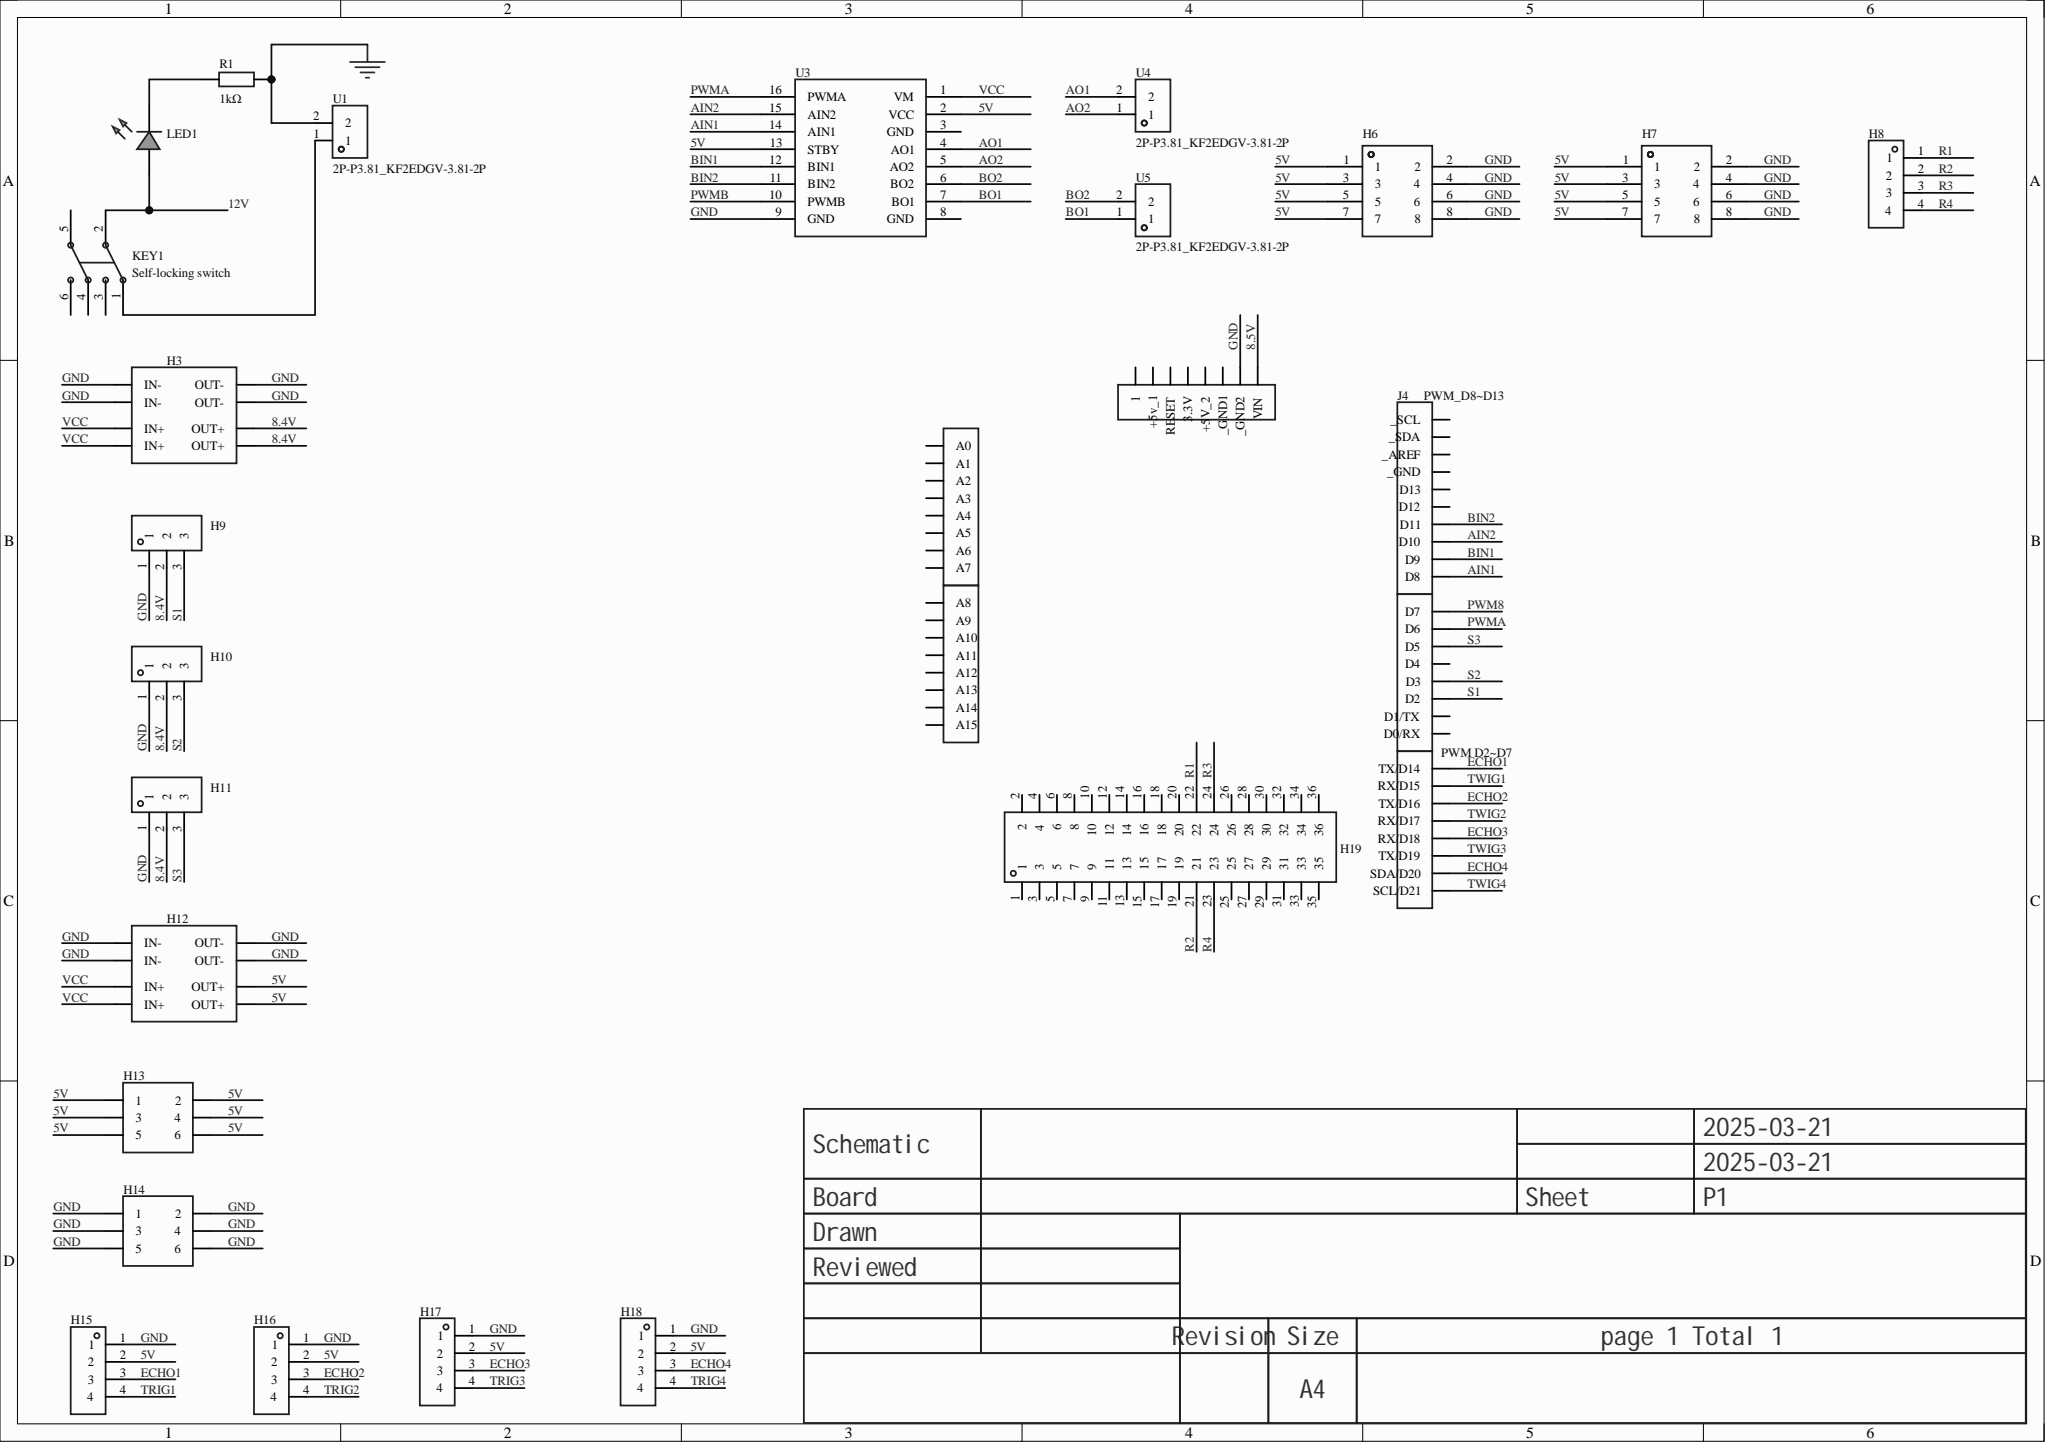Circuit board | Altium Designer | 28 parts | 27 nets
Bill of materials:
Comment,Description,Designator,Footprint,LibRef,Quantity
"","","H3, H12","HDR-TH_8P-P2.54-V-M","HDR-M_2.54_1x8P","2"
"","","H6, H7","HDR-TH_8P-P2.54-V-M-R2-C4-S2.54","HDR-M_2.54_2x4","2"
"","","H8","HDR-TH_4P-P2.54-V-F","HDR-F_2.54_1x4P","1"
"","","H9, H10, H11","HDR-TH_3P-P2.54-V-M","HDR-M_2.54_1x3P","3"
"","","H13, H14","HDR-TH_6P-P2.54-V-F-R2-C3-S2.54","HDR-F_2.54_2x3","2"
"","","H15, H16, H17, H18","HDR-TH_4P-P2.54-V-M","HDR-M_2.54_1x4P","4"
"X6521WV-2×18H-C30D60","","H19","HDR-TH_36P-2.54-V-M-R2-C18-S2.54","X6521WV-2×18H-C30D60","1"
"3-way TX/RX","","J1","HDR-M-2.54_1X8","3路TX/RX","1"
"PWM D2~D7","","J2","HDR-M-2.54_1X8","PWM D2~D7","1"
"PWM_D8~D13","","J4","HDR-M-2.54_1X10","PWM_D8~D13","1"
"HDR-M-2.54_1x8","","J8, J9, J14","HDR-M-2.54_1X8","HDR-M-2.54_1x8","3"
"Self-locking switch","","KEY1","SW-TH_6P-L8.5-W8.5-P2.54","无自锁开关 8.5×8.5 无声","1"
"","","LED1","LED_TH-3mm","LED_TH-G_3mm","1"
"1kΩ","","R1","Res_1/4W","Res_AXIAL-1/4W","1"
"2P-P3.81_KF2EDGV-3.81-2P","","U1, U4, U5","CONN-TH_2P-P3.81_KF2EDGV-3.81-2P","2P-P3.81_KF2EDGV-3.81-2P","3"
"tb6612","","U3","tb6612","tb6612","1"
Netlist (Protel format):
[
H3
HDR-TH_8P-P2.54-V-M




]
[
H6
HDR-TH_8P-P2.54-V-M-R2-C4-S2.54




]
[
H7
HDR-TH_8P-P2.54-V-M-R2-C4-S2.54




]
[
H8
HDR-TH_4P-P2.54-V-F




]
[
H9
HDR-TH_3P-P2.54-V-M




]
[
H10
HDR-TH_3P-P2.54-V-M




]
[
H11
HDR-TH_3P-P2.54-V-M




]
[
H12
HDR-TH_8P-P2.54-V-M




]
[
H13
HDR-TH_6P-P2.54-V-F-R2-C3-S2.54




]
[
H14
HDR-TH_6P-P2.54-V-F-R2-C3-S2.54




]
[
H15
HDR-TH_4P-P2.54-V-M




]
[
H16
HDR-TH_4P-P2.54-V-M




]
[
H17
HDR-TH_4P-P2.54-V-M




]
[
H18
HDR-TH_4P-P2.54-V-M




]
[
H19
HDR-TH_36P-2.54-V-M-R2-C18-S2.54
X6521WV-2×18H-C30D60



]
[
J1
HDR-M-2.54_1X8
3-way TX/RX



]
[
J2
HDR-M-2.54_1X8
PWM D2~D7



]
[
J4
HDR-M-2.54_1X10
PWM_D8~D13



]
[
J8
HDR-M-2.54_1X8
HDR-M-2.54_1x8



]
[
J9
HDR-M-2.54_1X8
HDR-M-2.54_1x8



]
[
J14
HDR-M-2.54_1X8
HDR-M-2.54_1x8



]
[
KEY1
SW-TH_6P-L8.5-W8.5-P2.54
Self-locking switch



]
[
LED1
LED_TH-3mm




]
[
R1
Res_1/4W
1kΩ



]
[
U1
CONN-TH_2P-P3.81_KF2EDGV-3.81-2P
2P-P3.81_KF2EDGV-3.81-2P



]
[
U3
tb6612
tb6612



]
[
U4
CONN-TH_2P-P3.81_KF2EDGV-3.81-2P
2P-P3.81_KF2EDGV-3.81-2P



]
[
U5
CONN-TH_2P-P3.81_KF2EDGV-3.81-2P
2P-P3.81_KF2EDGV-3.81-2P



]
(
VCC
H3-3
H3-4
H12-3
H12-4
U3-1
)
(
S3
H11-3
J2-3
)
(
S2
H10-3
J2-5
)
(
S1
H9-3
J2-6
)
(
R4
H8-4
H19-23
)
(
R3
H8-3
H19-24
)
(
R2
H8-2
H19-21
)
(
R1
H8-1
H19-22
)
(
PWMA
J2-2
U3-16
)
(
NetLED1_2
LED1-2
R1-1
)
(
NetKEY1_1
KEY1-1
U1-1
)
(
GND
H3-1
H3-2
H3-5
H3-6
H6-2
H6-4
H6-6
H6-8
H7-2
H7-4
H7-6
H7-8
H9-1
H10-1
H11-1
H12-1
H12-2
H12-5
H12-6
H14-1
H14-2
H14-3
H14-4
H14-5
H14-6
H15-1
H16-1
H17-1
H18-1
J9-7
R1-2
U1-2
U3-9
)
(
ECHO4
H18-3
J1-7
)
(
ECHO3
H17-3
J1-5
)
(
ECHO2
H16-3
J1-3
)
(
ECHO1
H15-3
J1-1
)
(
BO2
U3-6
U5-2
)
(
BO1
U3-7
U5-1
)
(
BIN2
J4-7
U3-11
)
(
BIN1
J4-9
U3-12
)
(
AO2
U3-5
U4-1
)
(
AO1
U3-4
U4-2
)
(
AIN2
J4-8
U3-15
)
(
AIN1
J4-10
U3-14
)
(
12V
KEY1-2
LED1-1
)
(
8.4V
H3-7
H3-8
H9-2
H10-2
H11-2
)
(
5V
H6-1
H6-3
H6-5
H6-7
H7-1
H7-3
H7-5
H7-7
H12-7
H12-8
H13-1
H13-2
H13-3
H13-4
H13-5
H13-6
H15-2
H16-2
H17-2
H18-2
U3-2
U3-13
)